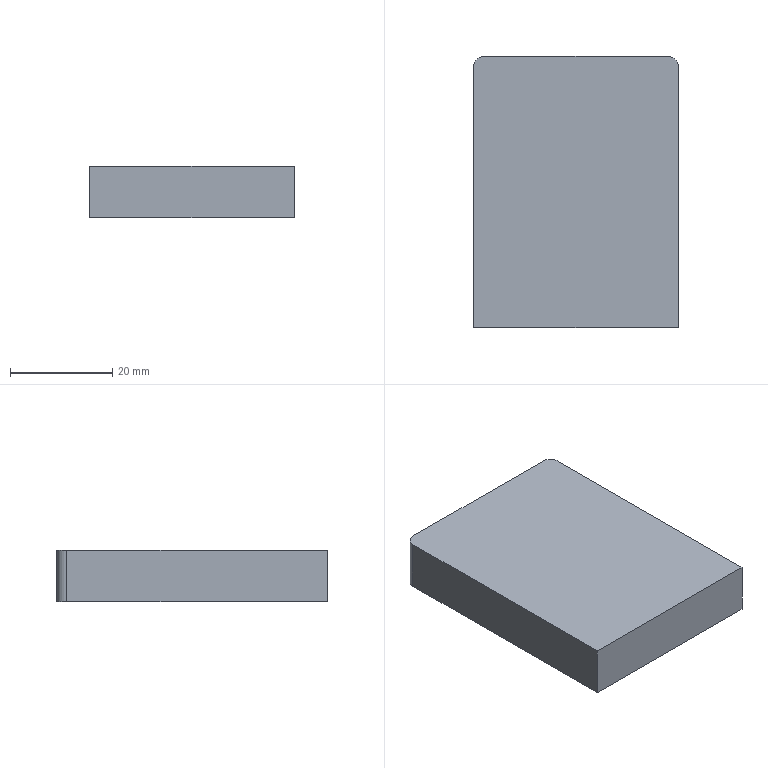Part | STEP file | SYL_0392D6J1SYL0380DJ10-1506056 | 1 solid | 8 faces | box 40 x 53 x 10 mm | volume 21183 mm3 | plane 6 | cylinder 2 | commonest cylinder face diameters 4 x2
STEP:
#1=CARTESIAN_POINT('',(-18.,53.,0.));
#2=VERTEX_POINT('',#1);
#3=CARTESIAN_POINT('',(-20.,51.,0.));
#4=VERTEX_POINT('',#3);
#5=CARTESIAN_POINT('',(-18.,51.,0.));
#6=DIRECTION('',(0.,0.,1.));
#7=DIRECTION('',(0.,1.,0.));
#8=AXIS2_PLACEMENT_3D('',#5,#6,#7);
#9=CIRCLE('',#8,2.);
#10=EDGE_CURVE('',#2,#4,#9,.T.);
#11=ORIENTED_EDGE('',*,*,#10,.T.);
#12=CARTESIAN_POINT('',(-20.,0.,0.));
#13=VERTEX_POINT('',#12);
#14=CARTESIAN_POINT('',(-20.,0.,0.));
#15=DIRECTION('',(0.,1.,0.));
#16=VECTOR('',#15,1000.);
#17=LINE('',#14,#16);
#18=EDGE_CURVE('',#13,#4,#17,.T.);
#19=ORIENTED_EDGE('',*,*,#18,.F.);
#20=CARTESIAN_POINT('',(20.,0.,0.));
#21=VERTEX_POINT('',#20);
#22=CARTESIAN_POINT('',(20.,0.,0.));
#23=DIRECTION('',(-1.,0.,0.));
#24=VECTOR('',#23,1000.);
#25=LINE('',#22,#24);
#26=EDGE_CURVE('',#21,#13,#25,.T.);
#27=ORIENTED_EDGE('',*,*,#26,.F.);
#28=CARTESIAN_POINT('',(20.,51.,0.));
#29=VERTEX_POINT('',#28);
#30=CARTESIAN_POINT('',(20.,51.,0.));
#31=DIRECTION('',(0.,-1.,0.));
#32=VECTOR('',#31,1000.);
#33=LINE('',#30,#32);
#34=EDGE_CURVE('',#29,#21,#33,.T.);
#35=ORIENTED_EDGE('',*,*,#34,.F.);
#36=CARTESIAN_POINT('',(18.,53.,0.));
#37=VERTEX_POINT('',#36);
#38=CARTESIAN_POINT('',(18.,51.,0.));
#39=DIRECTION('',(0.,0.,1.));
#40=DIRECTION('',(1.,0.,0.));
#41=AXIS2_PLACEMENT_3D('',#38,#39,#40);
#42=CIRCLE('',#41,2.);
#43=EDGE_CURVE('',#29,#37,#42,.T.);
#44=ORIENTED_EDGE('',*,*,#43,.T.);
#45=CARTESIAN_POINT('',(-18.,53.,0.));
#46=DIRECTION('',(1.,0.,0.));
#47=VECTOR('',#46,1000.);
#48=LINE('',#45,#47);
#49=EDGE_CURVE('',#2,#37,#48,.T.);
#50=ORIENTED_EDGE('',*,*,#49,.F.);
#51=EDGE_LOOP('',(#11,#19,#27,#35,#44,#50));
#52=FACE_OUTER_BOUND('',#51,.T.);
#53=CARTESIAN_POINT('',(0.,0.,0.));
#54=DIRECTION('',(0.,0.,1.));
#55=DIRECTION('',(1.,0.,0.));
#56=AXIS2_PLACEMENT_3D('',#53,#54,#55);
#57=PLANE('',#56);
#58=ADVANCED_FACE('',(#52),#57,.T.);
#59=CARTESIAN_POINT('',(20.,51.,-10.));
#60=VERTEX_POINT('',#59);
#61=CARTESIAN_POINT('',(20.,0.,-10.));
#62=VERTEX_POINT('',#61);
#63=CARTESIAN_POINT('',(20.,51.,-10.));
#64=DIRECTION('',(0.,-1.,0.));
#65=VECTOR('',#64,1000.);
#66=LINE('',#63,#65);
#67=EDGE_CURVE('',#60,#62,#66,.T.);
#68=ORIENTED_EDGE('',*,*,#67,.T.);
#69=CARTESIAN_POINT('',(-20.,0.,-10.));
#70=VERTEX_POINT('',#69);
#71=CARTESIAN_POINT('',(20.,0.,-10.));
#72=DIRECTION('',(-1.,0.,0.));
#73=VECTOR('',#72,1000.);
#74=LINE('',#71,#73);
#75=EDGE_CURVE('',#62,#70,#74,.T.);
#76=ORIENTED_EDGE('',*,*,#75,.T.);
#77=CARTESIAN_POINT('',(-20.,51.,-10.));
#78=VERTEX_POINT('',#77);
#79=CARTESIAN_POINT('',(-20.,0.,-10.));
#80=DIRECTION('',(0.,1.,0.));
#81=VECTOR('',#80,1000.);
#82=LINE('',#79,#81);
#83=EDGE_CURVE('',#70,#78,#82,.T.);
#84=ORIENTED_EDGE('',*,*,#83,.T.);
#85=CARTESIAN_POINT('',(-18.,53.,-10.));
#86=VERTEX_POINT('',#85);
#87=CARTESIAN_POINT('',(-18.,51.,-10.));
#88=DIRECTION('',(0.,0.,-1.));
#89=DIRECTION('',(-1.,0.,0.));
#90=AXIS2_PLACEMENT_3D('',#87,#88,#89);
#91=CIRCLE('',#90,2.);
#92=EDGE_CURVE('',#78,#86,#91,.T.);
#93=ORIENTED_EDGE('',*,*,#92,.T.);
#94=CARTESIAN_POINT('',(18.,53.,-10.));
#95=VERTEX_POINT('',#94);
#96=CARTESIAN_POINT('',(-18.,53.,-10.));
#97=DIRECTION('',(1.,0.,0.));
#98=VECTOR('',#97,1000.);
#99=LINE('',#96,#98);
#100=EDGE_CURVE('',#86,#95,#99,.T.);
#101=ORIENTED_EDGE('',*,*,#100,.T.);
#102=CARTESIAN_POINT('',(18.,51.,-10.));
#103=DIRECTION('',(0.,0.,-1.));
#104=DIRECTION('',(0.,1.,0.));
#105=AXIS2_PLACEMENT_3D('',#102,#103,#104);
#106=CIRCLE('',#105,2.);
#107=EDGE_CURVE('',#95,#60,#106,.T.);
#108=ORIENTED_EDGE('',*,*,#107,.T.);
#109=EDGE_LOOP('',(#68,#76,#84,#93,#101,#108));
#110=FACE_OUTER_BOUND('',#109,.T.);
#111=CARTESIAN_POINT('',(0.,0.,-10.));
#112=DIRECTION('',(0.,0.,1.));
#113=DIRECTION('',(1.,0.,0.));
#114=AXIS2_PLACEMENT_3D('',#111,#112,#113);
#115=PLANE('',#114);
#116=ADVANCED_FACE('',(#110),#115,.F.);
#117=ORIENTED_EDGE('',*,*,#18,.T.);
#118=CARTESIAN_POINT('',(-20.,51.,-10.));
#119=DIRECTION('',(0.,0.,1.));
#120=VECTOR('',#119,1000.);
#121=LINE('',#118,#120);
#122=EDGE_CURVE('',#78,#4,#121,.T.);
#123=ORIENTED_EDGE('',*,*,#122,.F.);
#124=ORIENTED_EDGE('',*,*,#83,.F.);
#125=CARTESIAN_POINT('',(-20.,0.,-10.));
#126=DIRECTION('',(0.,0.,1.));
#127=VECTOR('',#126,1000.);
#128=LINE('',#125,#127);
#129=EDGE_CURVE('',#70,#13,#128,.T.);
#130=ORIENTED_EDGE('',*,*,#129,.T.);
#131=EDGE_LOOP('',(#117,#123,#124,#130));
#132=FACE_OUTER_BOUND('',#131,.T.);
#133=CARTESIAN_POINT('',(-20.,25.5,-5.));
#134=DIRECTION('',(-1.,0.,0.));
#135=DIRECTION('',(0.,0.,1.));
#136=AXIS2_PLACEMENT_3D('',#133,#134,#135);
#137=PLANE('',#136);
#138=ADVANCED_FACE('',(#132),#137,.T.);
#139=ORIENTED_EDGE('',*,*,#10,.F.);
#140=CARTESIAN_POINT('',(-18.,53.,0.));
#141=DIRECTION('',(0.,0.,-1.));
#142=VECTOR('',#141,1000.);
#143=LINE('',#140,#142);
#144=EDGE_CURVE('',#2,#86,#143,.T.);
#145=ORIENTED_EDGE('',*,*,#144,.T.);
#146=ORIENTED_EDGE('',*,*,#92,.F.);
#147=ORIENTED_EDGE('',*,*,#122,.T.);
#148=EDGE_LOOP('',(#139,#145,#146,#147));
#149=FACE_OUTER_BOUND('',#148,.T.);
#150=CARTESIAN_POINT('',(-18.,51.,-5.));
#151=DIRECTION('',(0.,0.,1.));
#152=DIRECTION('',(1.,0.,0.));
#153=AXIS2_PLACEMENT_3D('',#150,#151,#152);
#154=CYLINDRICAL_SURFACE('',#153,2.);
#155=ADVANCED_FACE('',(#149),#154,.T.);
#156=ORIENTED_EDGE('',*,*,#49,.T.);
#157=CARTESIAN_POINT('',(18.,53.,-10.));
#158=DIRECTION('',(0.,0.,1.));
#159=VECTOR('',#158,1000.);
#160=LINE('',#157,#159);
#161=EDGE_CURVE('',#95,#37,#160,.T.);
#162=ORIENTED_EDGE('',*,*,#161,.F.);
#163=ORIENTED_EDGE('',*,*,#100,.F.);
#164=ORIENTED_EDGE('',*,*,#144,.F.);
#165=EDGE_LOOP('',(#156,#162,#163,#164));
#166=FACE_OUTER_BOUND('',#165,.T.);
#167=CARTESIAN_POINT('',(0.,53.,-5.));
#168=DIRECTION('',(0.,1.,0.));
#169=DIRECTION('',(1.,0.,0.));
#170=AXIS2_PLACEMENT_3D('',#167,#168,#169);
#171=PLANE('',#170);
#172=ADVANCED_FACE('',(#166),#171,.T.);
#173=ORIENTED_EDGE('',*,*,#43,.F.);
#174=CARTESIAN_POINT('',(20.,51.,0.));
#175=DIRECTION('',(0.,0.,-1.));
#176=VECTOR('',#175,1000.);
#177=LINE('',#174,#176);
#178=EDGE_CURVE('',#29,#60,#177,.T.);
#179=ORIENTED_EDGE('',*,*,#178,.T.);
#180=ORIENTED_EDGE('',*,*,#107,.F.);
#181=ORIENTED_EDGE('',*,*,#161,.T.);
#182=EDGE_LOOP('',(#173,#179,#180,#181));
#183=FACE_OUTER_BOUND('',#182,.T.);
#184=CARTESIAN_POINT('',(18.,51.,-5.));
#185=DIRECTION('',(0.,0.,1.));
#186=DIRECTION('',(1.,0.,0.));
#187=AXIS2_PLACEMENT_3D('',#184,#185,#186);
#188=CYLINDRICAL_SURFACE('',#187,2.);
#189=ADVANCED_FACE('',(#183),#188,.T.);
#190=ORIENTED_EDGE('',*,*,#34,.T.);
#191=CARTESIAN_POINT('',(20.,0.,-10.));
#192=DIRECTION('',(0.,0.,1.));
#193=VECTOR('',#192,1000.);
#194=LINE('',#191,#193);
#195=EDGE_CURVE('',#62,#21,#194,.T.);
#196=ORIENTED_EDGE('',*,*,#195,.F.);
#197=ORIENTED_EDGE('',*,*,#67,.F.);
#198=ORIENTED_EDGE('',*,*,#178,.F.);
#199=EDGE_LOOP('',(#190,#196,#197,#198));
#200=FACE_OUTER_BOUND('',#199,.T.);
#201=CARTESIAN_POINT('',(20.,25.5,-5.));
#202=DIRECTION('',(1.,0.,0.));
#203=DIRECTION('',(0.,1.,0.));
#204=AXIS2_PLACEMENT_3D('',#201,#202,#203);
#205=PLANE('',#204);
#206=ADVANCED_FACE('',(#200),#205,.T.);
#207=ORIENTED_EDGE('',*,*,#26,.T.);
#208=ORIENTED_EDGE('',*,*,#129,.F.);
#209=ORIENTED_EDGE('',*,*,#75,.F.);
#210=ORIENTED_EDGE('',*,*,#195,.T.);
#211=EDGE_LOOP('',(#207,#208,#209,#210));
#212=FACE_OUTER_BOUND('',#211,.T.);
#213=CARTESIAN_POINT('',(10.,0.,-5.));
#214=DIRECTION('',(0.,-1.,0.));
#215=DIRECTION('',(0.,0.,-1.));
#216=AXIS2_PLACEMENT_3D('',#213,#214,#215);
#217=PLANE('',#216);
#218=ADVANCED_FACE('',(#212),#217,.T.);
#219=CLOSED_SHELL('',(#58,#116,#138,#155,#172,#189,#206,#218));
#220=MANIFOLD_SOLID_BREP('',#219);
#221=CARTESIAN_POINT('',(0.,0.,0.));
#222=DIRECTION('',(0.,0.,1.));
#223=DIRECTION('',(1.,0.,0.));
#224=AXIS2_PLACEMENT_3D('',#221,#222,#223);
#225=(LENGTH_UNIT()NAMED_UNIT(*)SI_UNIT(.MILLI.,.METRE.));
#226=UNCERTAINTY_MEASURE_WITH_UNIT(LENGTH_MEASURE(0.00001),#225,'','');
#227=(NAMED_UNIT(*)PLANE_ANGLE_UNIT()SI_UNIT($,.RADIAN.));
#228=(NAMED_UNIT(*)SI_UNIT($,.STERADIAN.)SOLID_ANGLE_UNIT());
#229=(GEOMETRIC_REPRESENTATION_CONTEXT(3)GLOBAL_UNCERTAINTY_ASSIGNED_CONTEXT((#226))GLOBAL_UNIT_ASSIGNED_CONTEXT((#225,#227,#228))REPRESENTATION_CONTEXT('',''));
#230=ADVANCED_BREP_SHAPE_REPRESENTATION('',(#220,#224),#229);